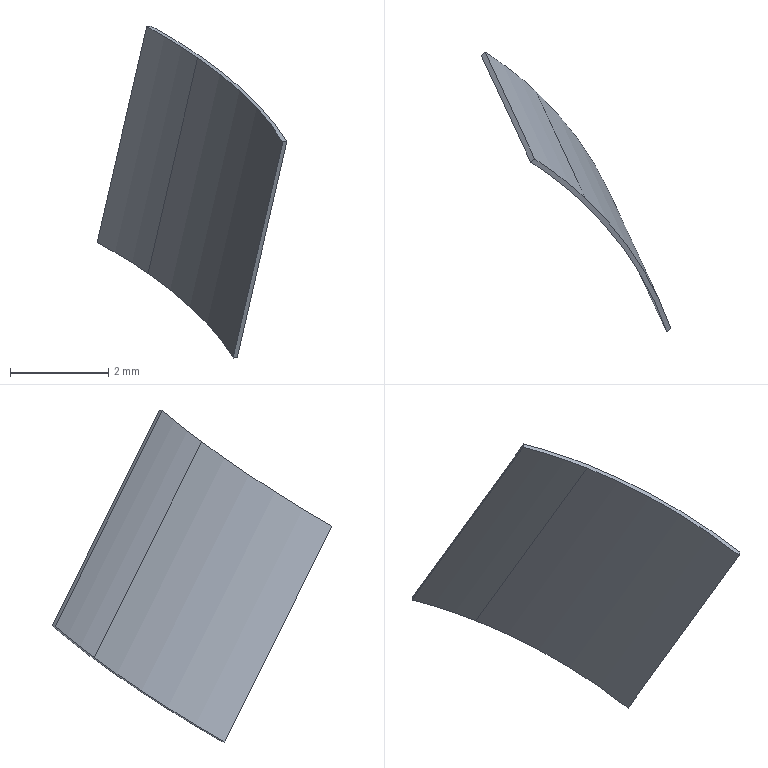Part | SolidWorks | features BaseBody 1 | 1 solid | 8 faces | box 3.855 x 5.685 x 6.743 mm | volume 2.538 mm3 | cylinder 4 | plane 4 | commonest cylinder face diameters 16.8 x2 17 x2
STEP:
#1=CARTESIAN_POINT('',(1973.205,-240.708,1002.032));
#2=VERTEX_POINT('',#1);
#3=CARTESIAN_POINT('',(1974.24,-241.505,1001.398));
#4=VERTEX_POINT('',#3);
#5=CARTESIAN_POINT('',(1968.101,-247.075,1000.039));
#6=DIRECTION('',(-0.2015,0.436,-0.8771));
#7=DIRECTION('',(-0.7309,-0.6631,-0.1618));
#8=AXIS2_PLACEMENT_3D('',#5,#6,#7);
#9=CIRCLE('',#8,8.4);
#10=EDGE_CURVE('',#2,#4,#9,.T.);
#11=ORIENTED_EDGE('',*,*,#10,.F.);
#12=CARTESIAN_POINT('',(1972.198,-238.528,997.647));
#13=VERTEX_POINT('',#12);
#14=CARTESIAN_POINT('',(1972.554,-239.299,999.199));
#15=DIRECTION('',(0.2015,-0.436,0.8771));
#16=VECTOR('',#15,1000.);
#17=LINE('',#14,#16);
#18=EDGE_CURVE('',#13,#2,#17,.T.);
#19=ORIENTED_EDGE('',*,*,#18,.F.);
#20=CARTESIAN_POINT('',(1973.233,-239.325,997.013));
#21=VERTEX_POINT('',#20);
#22=CARTESIAN_POINT('',(1967.093,-244.894,995.654));
#23=DIRECTION('',(0.2015,-0.436,0.8771));
#24=DIRECTION('',(-0.7309,-0.6631,-0.1618));
#25=AXIS2_PLACEMENT_3D('',#22,#23,#24);
#26=CIRCLE('',#25,8.4);
#27=EDGE_CURVE('',#21,#13,#26,.T.);
#28=ORIENTED_EDGE('',*,*,#27,.F.);
#29=CARTESIAN_POINT('',(1973.589,-240.097,998.565));
#30=DIRECTION('',(0.2015,-0.436,0.8771));
#31=VECTOR('',#30,1000.);
#32=LINE('',#29,#31);
#33=EDGE_CURVE('',#21,#4,#32,.T.);
#34=ORIENTED_EDGE('',*,*,#33,.T.);
#35=EDGE_LOOP('',(#11,#19,#28,#34));
#36=FACE_OUTER_BOUND('',#35,.T.);
#37=CARTESIAN_POINT('',(1967.45,-245.666,997.207));
#38=DIRECTION('',(0.2015,-0.436,0.8771));
#39=DIRECTION('',(-0.7309,-0.6631,-0.1618));
#40=AXIS2_PLACEMENT_3D('',#37,#38,#39);
#41=CYLINDRICAL_SURFACE('',#40,8.4);
#42=ADVANCED_FACE('',(#36),#41,.F.);
#43=CARTESIAN_POINT('',(1974.96,-241.971,995.3));
#44=VERTEX_POINT('',#43);
#45=CARTESIAN_POINT('',(1967.093,-244.894,995.654));
#46=DIRECTION('',(0.2015,-0.436,0.8771));
#47=DIRECTION('',(-0.7309,-0.6631,-0.1618));
#48=AXIS2_PLACEMENT_3D('',#45,#46,#47);
#49=CIRCLE('',#48,8.4);
#50=EDGE_CURVE('',#44,#21,#49,.T.);
#51=ORIENTED_EDGE('',*,*,#50,.F.);
#52=CARTESIAN_POINT('',(1975.968,-244.152,999.686));
#53=VERTEX_POINT('',#52);
#54=CARTESIAN_POINT('',(1975.317,-242.743,996.853));
#55=DIRECTION('',(-0.2015,0.436,-0.8771));
#56=VECTOR('',#55,1000.);
#57=LINE('',#54,#56);
#58=EDGE_CURVE('',#53,#44,#57,.T.);
#59=ORIENTED_EDGE('',*,*,#58,.F.);
#60=CARTESIAN_POINT('',(1968.101,-247.075,1000.039));
#61=DIRECTION('',(-0.2015,0.436,-0.8771));
#62=DIRECTION('',(-0.7309,-0.6631,-0.1618));
#63=AXIS2_PLACEMENT_3D('',#60,#61,#62);
#64=CIRCLE('',#63,8.4);
#65=EDGE_CURVE('',#4,#53,#64,.T.);
#66=ORIENTED_EDGE('',*,*,#65,.F.);
#67=ORIENTED_EDGE('',*,*,#33,.F.);
#68=EDGE_LOOP('',(#51,#59,#66,#67));
#69=FACE_OUTER_BOUND('',#68,.T.);
#70=CARTESIAN_POINT('',(1967.45,-245.666,997.207));
#71=DIRECTION('',(0.2015,-0.436,0.8771));
#72=DIRECTION('',(-0.7309,-0.6631,-0.1618));
#73=AXIS2_PLACEMENT_3D('',#70,#71,#72);
#74=CYLINDRICAL_SURFACE('',#73,8.4);
#75=ADVANCED_FACE('',(#69),#74,.F.);
#76=CARTESIAN_POINT('',(1973.306,-239.258,997.029));
#77=VERTEX_POINT('',#76);
#78=CARTESIAN_POINT('',(1972.282,-238.467,997.658));
#79=VERTEX_POINT('',#78);
#80=CARTESIAN_POINT('',(1967.093,-244.894,995.654));
#81=DIRECTION('',(0.2015,-0.436,0.8771));
#82=DIRECTION('',(-0.7309,-0.6631,-0.1618));
#83=AXIS2_PLACEMENT_3D('',#80,#81,#82);
#84=CIRCLE('',#83,8.5);
#85=EDGE_CURVE('',#77,#79,#84,.T.);
#86=ORIENTED_EDGE('',*,*,#85,.F.);
#87=CARTESIAN_POINT('',(1975.045,-241.911,995.311));
#88=VERTEX_POINT('',#87);
#89=CARTESIAN_POINT('',(1967.093,-244.894,995.654));
#90=DIRECTION('',(0.2015,-0.436,0.8771));
#91=DIRECTION('',(-0.7309,-0.6631,-0.1618));
#92=AXIS2_PLACEMENT_3D('',#89,#90,#91);
#93=CIRCLE('',#92,8.5);
#94=EDGE_CURVE('',#88,#77,#93,.T.);
#95=ORIENTED_EDGE('',*,*,#94,.F.);
#96=CARTESIAN_POINT('',(1975.003,-241.941,995.305));
#97=DIRECTION('',(-0.8088,-0.5792,-0.1022));
#98=VECTOR('',#97,1000.);
#99=LINE('',#96,#98);
#100=EDGE_CURVE('',#88,#44,#99,.T.);
#101=ORIENTED_EDGE('',*,*,#100,.T.);
#102=ORIENTED_EDGE('',*,*,#50,.T.);
#103=ORIENTED_EDGE('',*,*,#27,.T.);
#104=CARTESIAN_POINT('',(1972.24,-238.497,997.652));
#105=DIRECTION('',(-0.8088,-0.5792,-0.1022));
#106=VECTOR('',#105,1000.);
#107=LINE('',#104,#106);
#108=EDGE_CURVE('',#79,#13,#107,.T.);
#109=ORIENTED_EDGE('',*,*,#108,.F.);
#110=EDGE_LOOP('',(#86,#95,#101,#102,#103,#109));
#111=FACE_OUTER_BOUND('',#110,.T.);
#112=CARTESIAN_POINT('',(1980.606,-237.928,996.013));
#113=DIRECTION('',(0.2015,-0.436,0.8771));
#114=DIRECTION('',(0.5526,-0.6888,-0.4693));
#115=AXIS2_PLACEMENT_3D('',#112,#113,#114);
#116=PLANE('',#115);
#117=ADVANCED_FACE('',(#111),#116,.F.);
#118=CARTESIAN_POINT('',(1973.29,-240.647,1002.043));
#119=VERTEX_POINT('',#118);
#120=CARTESIAN_POINT('',(1972.786,-239.557,999.85));
#121=DIRECTION('',(0.2015,-0.436,0.8771));
#122=VECTOR('',#121,1000.);
#123=LINE('',#120,#122);
#124=EDGE_CURVE('',#79,#119,#123,.T.);
#125=ORIENTED_EDGE('',*,*,#124,.F.);
#126=ORIENTED_EDGE('',*,*,#108,.T.);
#127=ORIENTED_EDGE('',*,*,#18,.T.);
#128=CARTESIAN_POINT('',(1973.247,-240.678,1002.038));
#129=DIRECTION('',(-0.8088,-0.5792,-0.1022));
#130=VECTOR('',#129,1000.);
#131=LINE('',#128,#130);
#132=EDGE_CURVE('',#119,#2,#131,.T.);
#133=ORIENTED_EDGE('',*,*,#132,.F.);
#134=EDGE_LOOP('',(#125,#126,#127,#133));
#135=FACE_OUTER_BOUND('',#134,.T.);
#136=CARTESIAN_POINT('',(1977.843,-234.484,998.36));
#137=DIRECTION('',(0.5526,-0.6888,-0.4693));
#138=DIRECTION('',(-0.2015,0.436,-0.8771));
#139=AXIS2_PLACEMENT_3D('',#136,#137,#138);
#140=PLANE('',#139);
#141=ADVANCED_FACE('',(#135),#140,.F.);
#142=CARTESIAN_POINT('',(1974.313,-241.439,1001.414));
#143=VERTEX_POINT('',#142);
#144=CARTESIAN_POINT('',(1976.052,-244.091,999.696));
#145=VERTEX_POINT('',#144);
#146=CARTESIAN_POINT('',(1968.101,-247.075,1000.039));
#147=DIRECTION('',(-0.2015,0.436,-0.8771));
#148=DIRECTION('',(-0.7309,-0.6631,-0.1618));
#149=AXIS2_PLACEMENT_3D('',#146,#147,#148);
#150=CIRCLE('',#149,8.5);
#151=EDGE_CURVE('',#143,#145,#150,.T.);
#152=ORIENTED_EDGE('',*,*,#151,.F.);
#153=CARTESIAN_POINT('',(1968.101,-247.075,1000.039));
#154=DIRECTION('',(-0.2015,0.436,-0.8771));
#155=DIRECTION('',(-0.7309,-0.6631,-0.1618));
#156=AXIS2_PLACEMENT_3D('',#153,#154,#155);
#157=CIRCLE('',#156,8.5);
#158=EDGE_CURVE('',#119,#143,#157,.T.);
#159=ORIENTED_EDGE('',*,*,#158,.F.);
#160=ORIENTED_EDGE('',*,*,#132,.T.);
#161=ORIENTED_EDGE('',*,*,#10,.T.);
#162=ORIENTED_EDGE('',*,*,#65,.T.);
#163=CARTESIAN_POINT('',(1976.01,-244.121,999.691));
#164=DIRECTION('',(-0.8088,-0.5792,-0.1022));
#165=VECTOR('',#164,1000.);
#166=LINE('',#163,#165);
#167=EDGE_CURVE('',#145,#53,#166,.T.);
#168=ORIENTED_EDGE('',*,*,#167,.F.);
#169=EDGE_LOOP('',(#152,#159,#160,#161,#162,#168));
#170=FACE_OUTER_BOUND('',#169,.T.);
#171=CARTESIAN_POINT('',(1978.851,-236.665,1002.746));
#172=DIRECTION('',(-0.2015,0.436,-0.8771));
#173=DIRECTION('',(-0.5526,0.6888,0.4693));
#174=AXIS2_PLACEMENT_3D('',#171,#172,#173);
#175=PLANE('',#174);
#176=ADVANCED_FACE('',(#170),#175,.F.);
#177=CARTESIAN_POINT('',(1975.549,-243.001,997.504));
#178=DIRECTION('',(-0.2015,0.436,-0.8771));
#179=VECTOR('',#178,1000.);
#180=LINE('',#177,#179);
#181=EDGE_CURVE('',#145,#88,#180,.T.);
#182=ORIENTED_EDGE('',*,*,#181,.F.);
#183=ORIENTED_EDGE('',*,*,#167,.T.);
#184=ORIENTED_EDGE('',*,*,#58,.T.);
#185=ORIENTED_EDGE('',*,*,#100,.F.);
#186=EDGE_LOOP('',(#182,#183,#184,#185));
#187=FACE_OUTER_BOUND('',#186,.T.);
#188=CARTESIAN_POINT('',(1981.613,-240.108,1000.399));
#189=DIRECTION('',(-0.5526,0.6888,0.4693));
#190=DIRECTION('',(0.2015,-0.436,0.8771));
#191=AXIS2_PLACEMENT_3D('',#188,#189,#190);
#192=PLANE('',#191);
#193=ADVANCED_FACE('',(#187),#192,.F.);
#194=CARTESIAN_POINT('',(1973.662,-240.03,998.581));
#195=DIRECTION('',(0.2015,-0.436,0.8771));
#196=VECTOR('',#195,1000.);
#197=LINE('',#194,#196);
#198=EDGE_CURVE('',#77,#143,#197,.T.);
#199=ORIENTED_EDGE('',*,*,#198,.F.);
#200=ORIENTED_EDGE('',*,*,#85,.T.);
#201=ORIENTED_EDGE('',*,*,#124,.T.);
#202=ORIENTED_EDGE('',*,*,#158,.T.);
#203=EDGE_LOOP('',(#199,#200,#201,#202));
#204=FACE_OUTER_BOUND('',#203,.T.);
#205=CARTESIAN_POINT('',(1967.45,-245.666,997.207));
#206=DIRECTION('',(0.2015,-0.436,0.8771));
#207=DIRECTION('',(-0.7309,-0.6631,-0.1618));
#208=AXIS2_PLACEMENT_3D('',#205,#206,#207);
#209=CYLINDRICAL_SURFACE('',#208,8.5);
#210=ADVANCED_FACE('',(#204),#209,.T.);
#211=ORIENTED_EDGE('',*,*,#198,.T.);
#212=ORIENTED_EDGE('',*,*,#151,.T.);
#213=ORIENTED_EDGE('',*,*,#181,.T.);
#214=ORIENTED_EDGE('',*,*,#94,.T.);
#215=EDGE_LOOP('',(#211,#212,#213,#214));
#216=FACE_OUTER_BOUND('',#215,.T.);
#217=CARTESIAN_POINT('',(1967.45,-245.666,997.207));
#218=DIRECTION('',(0.2015,-0.436,0.8771));
#219=DIRECTION('',(-0.7309,-0.6631,-0.1618));
#220=AXIS2_PLACEMENT_3D('',#217,#218,#219);
#221=CYLINDRICAL_SURFACE('',#220,8.5);
#222=ADVANCED_FACE('',(#216),#221,.T.);
#223=CLOSED_SHELL('',(#42,#75,#117,#141,#176,#193,#210,#222));
#224=MANIFOLD_SOLID_BREP('',#223);
#225=CARTESIAN_POINT('',(0.,0.,0.));
#226=DIRECTION('',(0.,0.,1.));
#227=DIRECTION('',(1.,0.,0.));
#228=AXIS2_PLACEMENT_3D('',#225,#226,#227);
#229=(LENGTH_UNIT()NAMED_UNIT(*)SI_UNIT(.MILLI.,.METRE.));
#230=UNCERTAINTY_MEASURE_WITH_UNIT(LENGTH_MEASURE(0.00001),#229,'','');
#231=(NAMED_UNIT(*)PLANE_ANGLE_UNIT()SI_UNIT($,.RADIAN.));
#232=(NAMED_UNIT(*)SI_UNIT($,.STERADIAN.)SOLID_ANGLE_UNIT());
#233=(GEOMETRIC_REPRESENTATION_CONTEXT(3)GLOBAL_UNCERTAINTY_ASSIGNED_CONTEXT((#230))GLOBAL_UNIT_ASSIGNED_CONTEXT((#229,#231,#232))REPRESENTATION_CONTEXT('',''));
#234=ADVANCED_BREP_SHAPE_REPRESENTATION('',(#224,#228),#233);